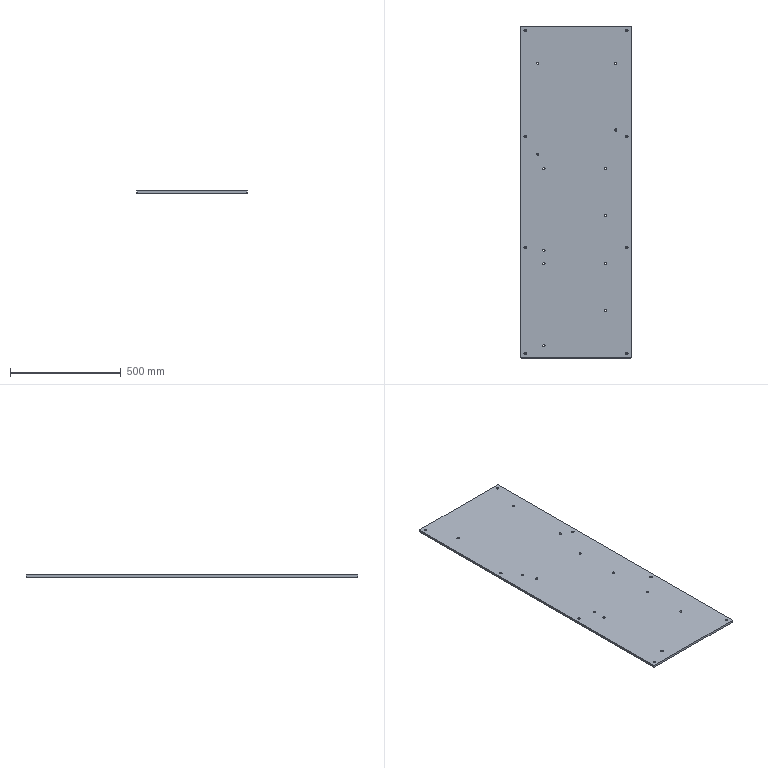Part | STEP file | 1 solid | 74 faces | box 500 x 1500 x 10 mm | volume 7485180 mm3 | cylinder 60 | plane 14 | commonest cylinder face diameters 10.2 x24 6.5 x16 11 x16 4 x4